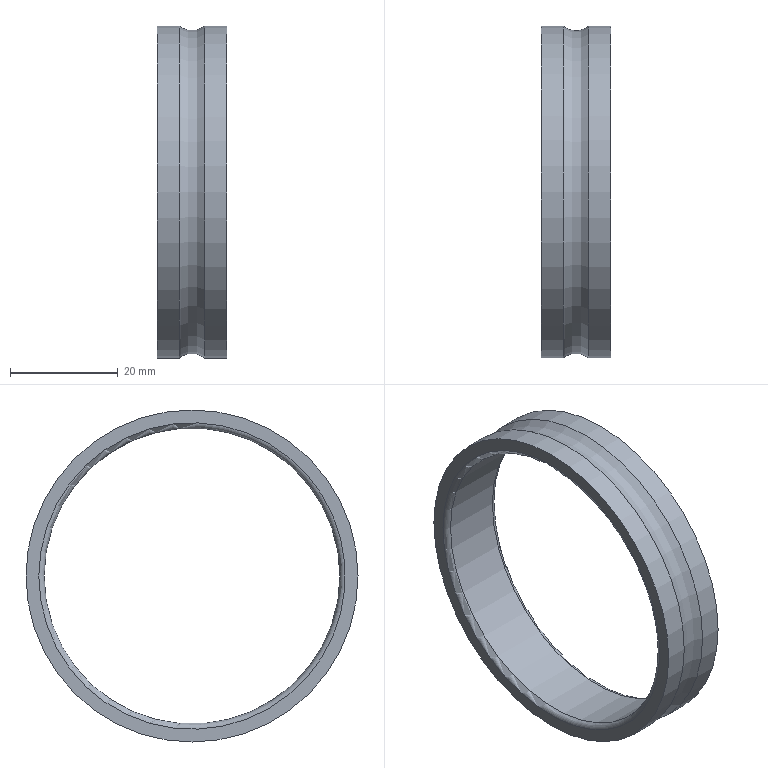Part | STEP file | Inner ring | 1 solid | 8 faces | box 13 x 61.75 x 61.75 mm | volume 7419 mm3 | cylinder 3 | torus 3 | plane 2 | commonest cylinder face diameters 61.75 x2 55 x1
STEP:
#1=CARTESIAN_POINT('',(6.5,30.875,0.));
#2=VERTEX_POINT('',#1);
#3=CARTESIAN_POINT('',(6.5,0.,0.));
#4=DIRECTION('',(1.,0.,0.));
#5=DIRECTION('',(0.,1.,0.));
#6=AXIS2_PLACEMENT_3D('',#3,#4,#5);
#7=CIRCLE('',#6,30.875);
#8=EDGE_CURVE('',#2,#2,#7,.T.);
#9=ORIENTED_EDGE('',*,*,#8,.F.);
#10=EDGE_LOOP('',(#9));
#11=FACE_OUTER_BOUND('',#10,.T.);
#12=CARTESIAN_POINT('',(2.408,30.875,0.));
#13=VERTEX_POINT('',#12);
#14=CARTESIAN_POINT('',(2.408,0.,0.));
#15=DIRECTION('',(1.,0.,0.));
#16=DIRECTION('',(0.,1.,0.));
#17=AXIS2_PLACEMENT_3D('',#14,#15,#16);
#18=CIRCLE('',#17,30.875);
#19=EDGE_CURVE('',#13,#13,#18,.T.);
#20=ORIENTED_EDGE('',*,*,#19,.T.);
#21=EDGE_LOOP('',(#20));
#22=FACE_OUTER_BOUND('',#21,.T.);
#23=CARTESIAN_POINT('',(-6.5,0.,0.));
#24=DIRECTION('',(1.,0.,0.));
#25=DIRECTION('',(0.,1.,0.));
#26=AXIS2_PLACEMENT_3D('',#23,#24,#25);
#27=CYLINDRICAL_SURFACE('',#26,30.875);
#28=ADVANCED_FACE('',(#11,#22),#27,.T.);
#29=CARTESIAN_POINT('',(-2.408,30.875,0.));
#30=VERTEX_POINT('',#29);
#31=CARTESIAN_POINT('',(-2.408,0.,0.));
#32=DIRECTION('',(1.,0.,0.));
#33=DIRECTION('',(0.,1.,0.));
#34=AXIS2_PLACEMENT_3D('',#31,#32,#33);
#35=CIRCLE('',#34,30.875);
#36=EDGE_CURVE('',#30,#30,#35,.F.);
#37=ORIENTED_EDGE('',*,*,#36,.T.);
#38=EDGE_LOOP('',(#37));
#39=FACE_OUTER_BOUND('',#38,.T.);
#40=CARTESIAN_POINT('',(-6.5,30.875,0.));
#41=VERTEX_POINT('',#40);
#42=CARTESIAN_POINT('',(-6.5,0.,0.));
#43=DIRECTION('',(1.,0.,0.));
#44=DIRECTION('',(0.,1.,0.));
#45=AXIS2_PLACEMENT_3D('',#42,#43,#44);
#46=CIRCLE('',#45,30.875);
#47=EDGE_CURVE('',#41,#41,#46,.T.);
#48=ORIENTED_EDGE('',*,*,#47,.T.);
#49=EDGE_LOOP('',(#48));
#50=FACE_OUTER_BOUND('',#49,.T.);
#51=CARTESIAN_POINT('',(-6.5,0.,0.));
#52=DIRECTION('',(1.,0.,0.));
#53=DIRECTION('',(0.,1.,0.));
#54=AXIS2_PLACEMENT_3D('',#51,#52,#53);
#55=CYLINDRICAL_SURFACE('',#54,30.875);
#56=ADVANCED_FACE('',(#39,#50),#55,.T.);
#57=ORIENTED_EDGE('',*,*,#19,.F.);
#58=EDGE_LOOP('',(#57));
#59=FACE_OUTER_BOUND('',#58,.T.);
#60=ORIENTED_EDGE('',*,*,#36,.F.);
#61=EDGE_LOOP('',(#60));
#62=FACE_OUTER_BOUND('',#61,.T.);
#63=CARTESIAN_POINT('',(0.,0.,0.));
#64=DIRECTION('',(1.,0.,0.));
#65=DIRECTION('',(0.,1.,0.));
#66=AXIS2_PLACEMENT_3D('',#63,#64,#65);
#67=TOROIDAL_SURFACE('',#66,33.75,3.75);
#68=ADVANCED_FACE('',(#59,#62),#67,.F.);
#69=ORIENTED_EDGE('',*,*,#8,.T.);
#70=EDGE_LOOP('',(#69));
#71=FACE_BOUND('',#70,.T.);
#72=CARTESIAN_POINT('',(6.5,28.5,0.));
#73=VERTEX_POINT('',#72);
#74=CARTESIAN_POINT('',(6.5,0.,0.));
#75=DIRECTION('',(1.,0.,0.));
#76=DIRECTION('',(0.,1.,0.));
#77=AXIS2_PLACEMENT_3D('',#74,#75,#76);
#78=CIRCLE('',#77,28.5);
#79=EDGE_CURVE('',#73,#73,#78,.T.);
#80=ORIENTED_EDGE('',*,*,#79,.F.);
#81=EDGE_LOOP('',(#80));
#82=FACE_BOUND('',#81,.T.);
#83=CARTESIAN_POINT('',(6.5,0.,0.));
#84=DIRECTION('',(1.,0.,0.));
#85=DIRECTION('',(0.,1.,0.));
#86=AXIS2_PLACEMENT_3D('',#83,#84,#85);
#87=PLANE('',#86);
#88=ADVANCED_FACE('',(#71,#82),#87,.T.);
#89=ORIENTED_EDGE('',*,*,#47,.F.);
#90=EDGE_LOOP('',(#89));
#91=FACE_BOUND('',#90,.T.);
#92=CARTESIAN_POINT('',(-6.5,28.5,0.));
#93=VERTEX_POINT('',#92);
#94=CARTESIAN_POINT('',(-6.5,0.,0.));
#95=DIRECTION('',(1.,0.,0.));
#96=DIRECTION('',(0.,1.,0.));
#97=AXIS2_PLACEMENT_3D('',#94,#95,#96);
#98=CIRCLE('',#97,28.5);
#99=EDGE_CURVE('',#93,#93,#98,.T.);
#100=ORIENTED_EDGE('',*,*,#99,.T.);
#101=EDGE_LOOP('',(#100));
#102=FACE_BOUND('',#101,.T.);
#103=CARTESIAN_POINT('',(-6.5,0.,0.));
#104=DIRECTION('',(-1.,0.,0.));
#105=DIRECTION('',(0.,1.,0.));
#106=AXIS2_PLACEMENT_3D('',#103,#104,#105);
#107=PLANE('',#106);
#108=ADVANCED_FACE('',(#91,#102),#107,.T.);
#109=CARTESIAN_POINT('',(5.5,27.5,0.));
#110=VERTEX_POINT('',#109);
#111=CARTESIAN_POINT('',(5.5,0.,0.));
#112=DIRECTION('',(1.,0.,0.));
#113=DIRECTION('',(0.,1.,0.));
#114=AXIS2_PLACEMENT_3D('',#111,#112,#113);
#115=CIRCLE('',#114,27.5);
#116=EDGE_CURVE('',#110,#110,#115,.T.);
#117=ORIENTED_EDGE('',*,*,#116,.T.);
#118=EDGE_LOOP('',(#117));
#119=FACE_OUTER_BOUND('',#118,.T.);
#120=CARTESIAN_POINT('',(-5.5,27.5,0.));
#121=VERTEX_POINT('',#120);
#122=CARTESIAN_POINT('',(-5.5,0.,0.));
#123=DIRECTION('',(1.,0.,0.));
#124=DIRECTION('',(0.,1.,0.));
#125=AXIS2_PLACEMENT_3D('',#122,#123,#124);
#126=CIRCLE('',#125,27.5);
#127=EDGE_CURVE('',#121,#121,#126,.T.);
#128=ORIENTED_EDGE('',*,*,#127,.F.);
#129=EDGE_LOOP('',(#128));
#130=FACE_OUTER_BOUND('',#129,.T.);
#131=CARTESIAN_POINT('',(6.5,0.,0.));
#132=DIRECTION('',(1.,0.,0.));
#133=DIRECTION('',(0.,1.,0.));
#134=AXIS2_PLACEMENT_3D('',#131,#132,#133);
#135=CYLINDRICAL_SURFACE('',#134,27.5);
#136=ADVANCED_FACE('',(#119,#130),#135,.F.);
#137=ORIENTED_EDGE('',*,*,#127,.T.);
#138=EDGE_LOOP('',(#137));
#139=FACE_OUTER_BOUND('',#138,.T.);
#140=ORIENTED_EDGE('',*,*,#99,.F.);
#141=EDGE_LOOP('',(#140));
#142=FACE_OUTER_BOUND('',#141,.T.);
#143=CARTESIAN_POINT('',(-5.5,0.,0.));
#144=DIRECTION('',(1.,0.,0.));
#145=DIRECTION('',(0.,1.,0.));
#146=AXIS2_PLACEMENT_3D('',#143,#144,#145);
#147=TOROIDAL_SURFACE('',#146,28.5,1.);
#148=ADVANCED_FACE('',(#139,#142),#147,.T.);
#149=ORIENTED_EDGE('',*,*,#79,.T.);
#150=EDGE_LOOP('',(#149));
#151=FACE_OUTER_BOUND('',#150,.T.);
#152=ORIENTED_EDGE('',*,*,#116,.F.);
#153=EDGE_LOOP('',(#152));
#154=FACE_OUTER_BOUND('',#153,.T.);
#155=CARTESIAN_POINT('',(5.5,0.,0.));
#156=DIRECTION('',(1.,0.,0.));
#157=DIRECTION('',(0.,1.,0.));
#158=AXIS2_PLACEMENT_3D('',#155,#156,#157);
#159=TOROIDAL_SURFACE('',#158,28.5,1.);
#160=ADVANCED_FACE('',(#151,#154),#159,.T.);
#161=CLOSED_SHELL('',(#28,#56,#68,#88,#108,#136,#148,#160));
#162=MANIFOLD_SOLID_BREP('',#161);
#163=(LENGTH_UNIT()NAMED_UNIT(*)SI_UNIT(.MILLI.,.METRE.));
#164=UNCERTAINTY_MEASURE_WITH_UNIT(LENGTH_MEASURE(0.00001),#163,'','');
#165=(NAMED_UNIT(*)PLANE_ANGLE_UNIT()SI_UNIT($,.RADIAN.));
#166=(NAMED_UNIT(*)SI_UNIT($,.STERADIAN.)SOLID_ANGLE_UNIT());
#167=(GEOMETRIC_REPRESENTATION_CONTEXT(3)GLOBAL_UNCERTAINTY_ASSIGNED_CONTEXT((#164))GLOBAL_UNIT_ASSIGNED_CONTEXT((#163,#165,#166))REPRESENTATION_CONTEXT('',''));
#168=ADVANCED_BREP_SHAPE_REPRESENTATION('',(#162),#167);